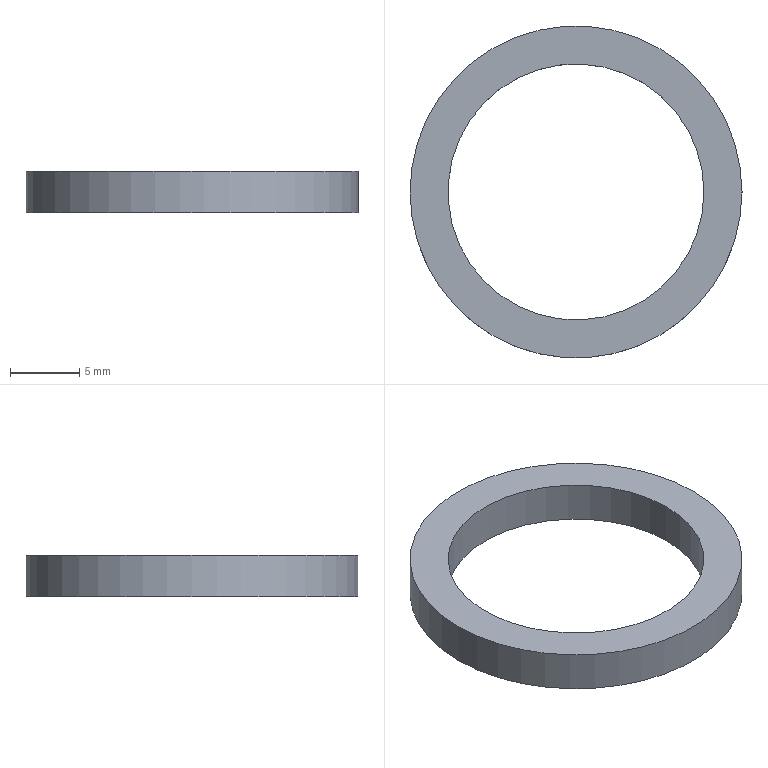Part | NX | features DATUM_CSYS 2, EXTRUDE 1, SKETCH 1 | 1 solid | 4 faces | box 24 x 24 x 3 mm | volume 550.76 mm3 | cylinder 2 | plane 2 | commonest cylinder face diameters 18.5 x1 24 x1
STEP:
#1=CARTESIAN_POINT('',(12.,0.,3.));
#2=VERTEX_POINT('',#1);
#3=CARTESIAN_POINT('',(0.,0.,3.));
#4=DIRECTION('',(0.,0.,1.));
#5=DIRECTION('',(1.,0.,0.));
#6=AXIS2_PLACEMENT_3D('',#3,#4,#5);
#7=CIRCLE('',#6,12.);
#8=EDGE_CURVE('',#2,#2,#7,.T.);
#9=ORIENTED_EDGE('',*,*,#8,.F.);
#10=EDGE_LOOP('',(#9));
#11=FACE_BOUND('',#10,.T.);
#12=CARTESIAN_POINT('',(12.,0.,0.));
#13=VERTEX_POINT('',#12);
#14=CARTESIAN_POINT('',(0.,0.,0.));
#15=DIRECTION('',(0.,0.,1.));
#16=DIRECTION('',(1.,0.,0.));
#17=AXIS2_PLACEMENT_3D('',#14,#15,#16);
#18=CIRCLE('',#17,12.);
#19=EDGE_CURVE('',#13,#13,#18,.T.);
#20=ORIENTED_EDGE('',*,*,#19,.T.);
#21=EDGE_LOOP('',(#20));
#22=FACE_BOUND('',#21,.T.);
#23=CARTESIAN_POINT('',(0.,0.,3.));
#24=DIRECTION('',(0.,0.,-1.));
#25=DIRECTION('',(-1.,0.,0.));
#26=AXIS2_PLACEMENT_3D('',#23,#24,#25);
#27=CYLINDRICAL_SURFACE('',#26,12.);
#28=ADVANCED_FACE('',(#11,#22),#27,.T.);
#29=CARTESIAN_POINT('',(9.25,0.,3.));
#30=VERTEX_POINT('',#29);
#31=CARTESIAN_POINT('',(0.,0.,3.));
#32=DIRECTION('',(0.,0.,1.));
#33=DIRECTION('',(1.,0.,0.));
#34=AXIS2_PLACEMENT_3D('',#31,#32,#33);
#35=CIRCLE('',#34,9.25);
#36=EDGE_CURVE('',#30,#30,#35,.T.);
#37=ORIENTED_EDGE('',*,*,#36,.T.);
#38=EDGE_LOOP('',(#37));
#39=FACE_BOUND('',#38,.T.);
#40=CARTESIAN_POINT('',(9.25,0.,0.));
#41=VERTEX_POINT('',#40);
#42=CARTESIAN_POINT('',(0.,0.,0.));
#43=DIRECTION('',(0.,0.,1.));
#44=DIRECTION('',(1.,0.,0.));
#45=AXIS2_PLACEMENT_3D('',#42,#43,#44);
#46=CIRCLE('',#45,9.25);
#47=EDGE_CURVE('',#41,#41,#46,.T.);
#48=ORIENTED_EDGE('',*,*,#47,.F.);
#49=EDGE_LOOP('',(#48));
#50=FACE_BOUND('',#49,.T.);
#51=CARTESIAN_POINT('',(0.,0.,3.));
#52=DIRECTION('',(0.,0.,-1.));
#53=DIRECTION('',(-1.,0.,0.));
#54=AXIS2_PLACEMENT_3D('',#51,#52,#53);
#55=CYLINDRICAL_SURFACE('',#54,9.25);
#56=ADVANCED_FACE('',(#39,#50),#55,.F.);
#57=ORIENTED_EDGE('',*,*,#8,.T.);
#58=EDGE_LOOP('',(#57));
#59=FACE_BOUND('',#58,.T.);
#60=ORIENTED_EDGE('',*,*,#36,.F.);
#61=EDGE_LOOP('',(#60));
#62=FACE_BOUND('',#61,.T.);
#63=CARTESIAN_POINT('',(0.,0.,3.));
#64=DIRECTION('',(0.,0.,1.));
#65=DIRECTION('',(1.,0.,0.));
#66=AXIS2_PLACEMENT_3D('',#63,#64,#65);
#67=PLANE('',#66);
#68=ADVANCED_FACE('',(#59,#62),#67,.T.);
#69=ORIENTED_EDGE('',*,*,#19,.F.);
#70=EDGE_LOOP('',(#69));
#71=FACE_BOUND('',#70,.T.);
#72=ORIENTED_EDGE('',*,*,#47,.T.);
#73=EDGE_LOOP('',(#72));
#74=FACE_BOUND('',#73,.T.);
#75=CARTESIAN_POINT('',(0.,0.,0.));
#76=DIRECTION('',(0.,0.,1.));
#77=DIRECTION('',(1.,0.,0.));
#78=AXIS2_PLACEMENT_3D('',#75,#76,#77);
#79=PLANE('',#78);
#80=ADVANCED_FACE('',(#71,#74),#79,.F.);
#81=CLOSED_SHELL('',(#28,#56,#68,#80));
#82=MANIFOLD_SOLID_BREP('',#81);
#83=(LENGTH_UNIT()NAMED_UNIT(*)SI_UNIT(.MILLI.,.METRE.));
#84=UNCERTAINTY_MEASURE_WITH_UNIT(LENGTH_MEASURE(0.00001),#83,'','');
#85=(NAMED_UNIT(*)PLANE_ANGLE_UNIT()SI_UNIT($,.RADIAN.));
#86=(NAMED_UNIT(*)SI_UNIT($,.STERADIAN.)SOLID_ANGLE_UNIT());
#87=(GEOMETRIC_REPRESENTATION_CONTEXT(3)GLOBAL_UNCERTAINTY_ASSIGNED_CONTEXT((#84))GLOBAL_UNIT_ASSIGNED_CONTEXT((#83,#85,#86))REPRESENTATION_CONTEXT('',''));
#88=ADVANCED_BREP_SHAPE_REPRESENTATION('',(#82),#87);